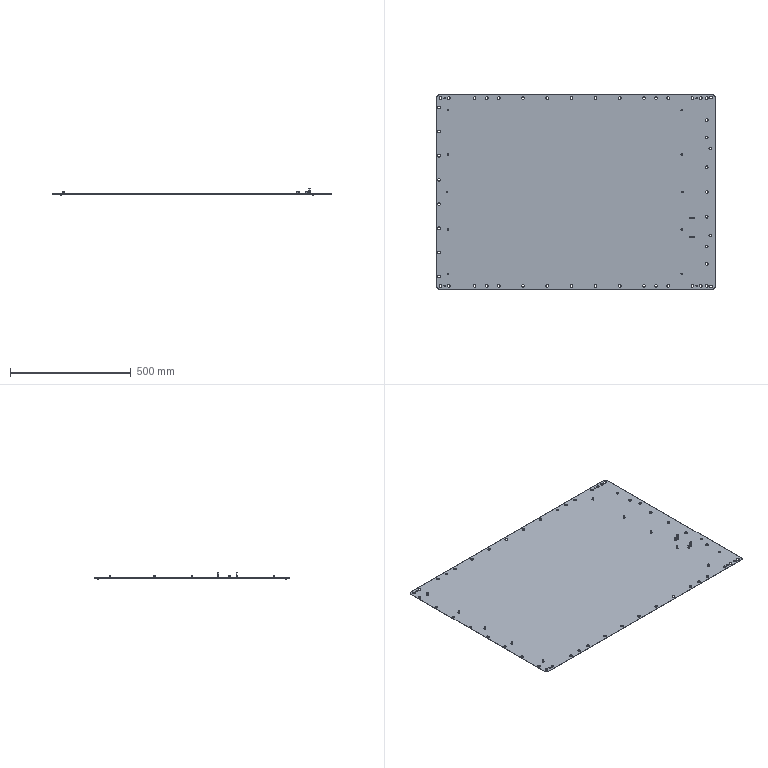Part | NX | features BREP 7 | 19 solids | 474 faces | box 1150 x 803 x 25.8 mm | volume 1105685 mm3 | cylinder 218 | plane 192 | cone 64 | commonest cylinder face diameters 11 x94 3.2 x32 5.95 x28 6 x28 4 x8 4.1 x8